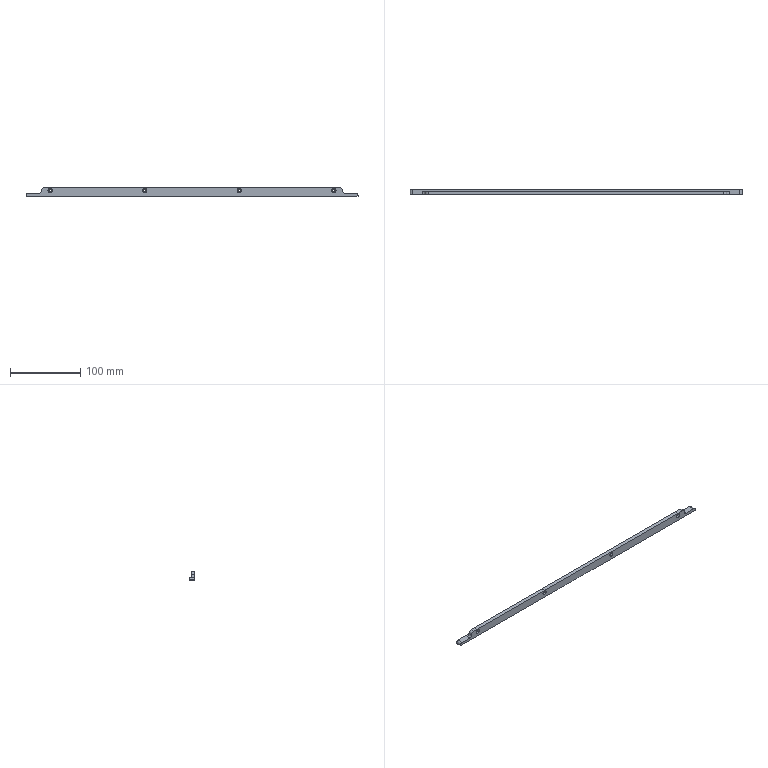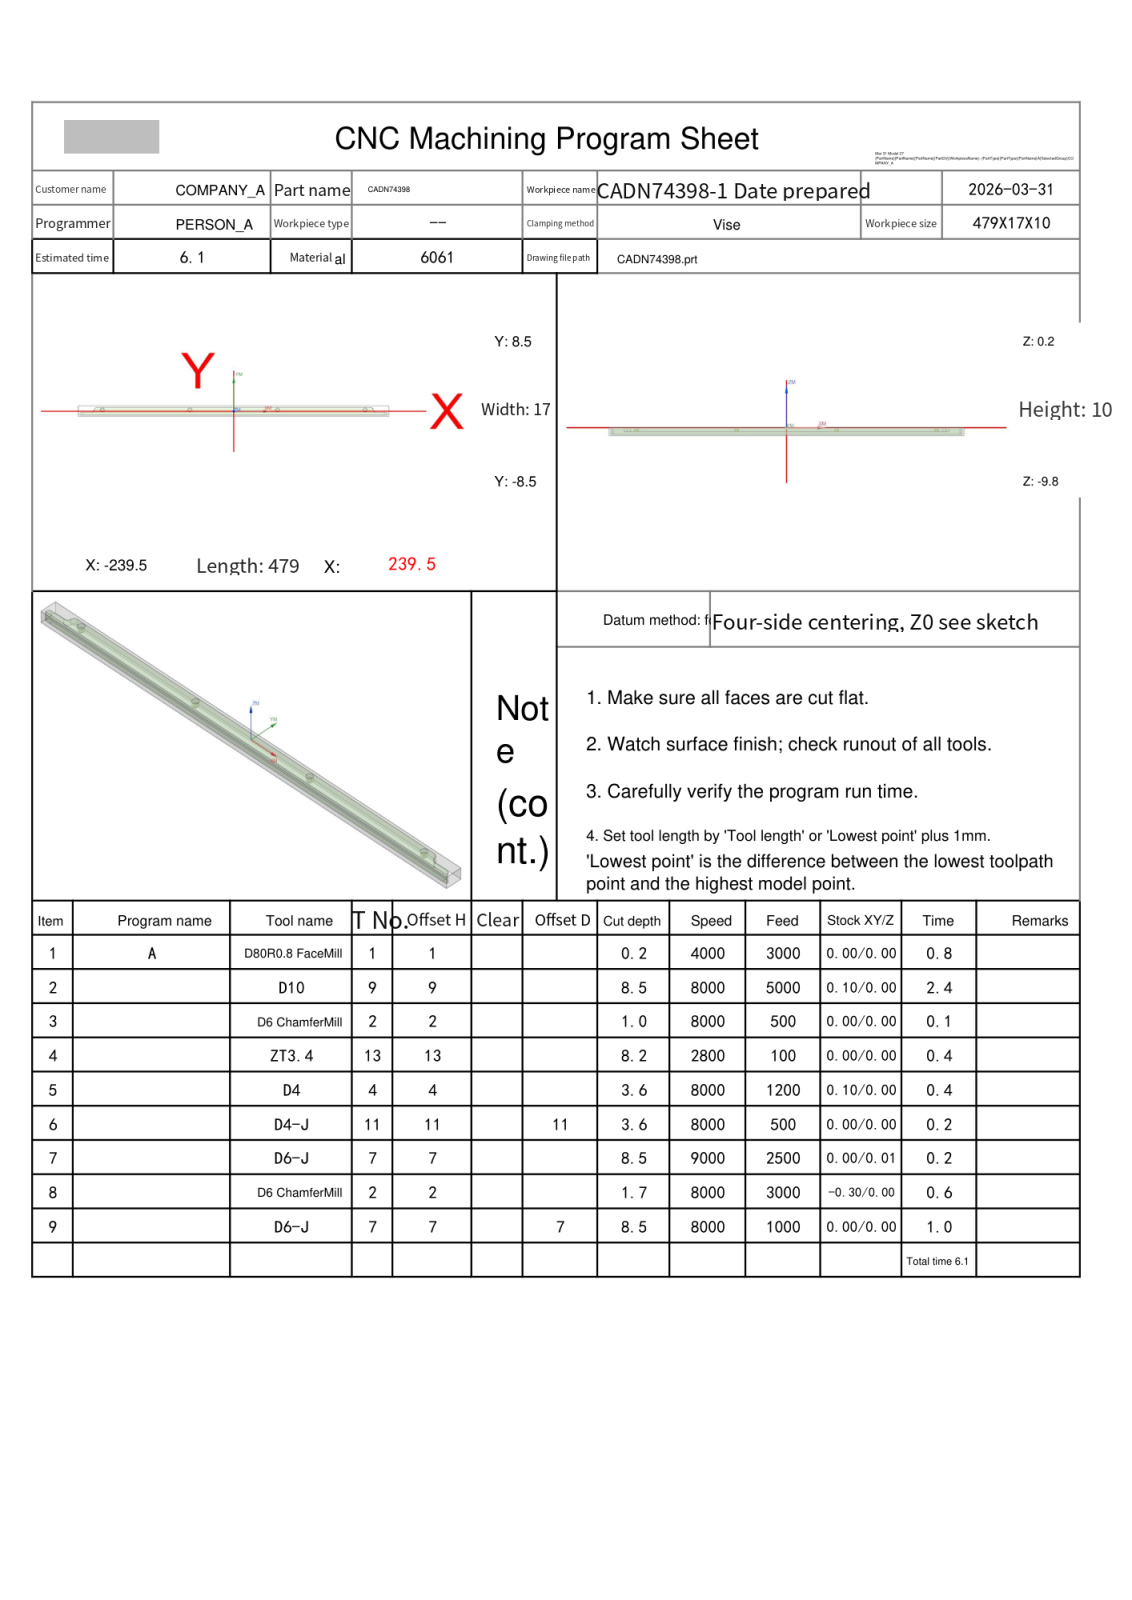NC program | NX | posted by the shop | part box 474 x 8.3 x 12 mm
Lines 413 to 2396 of 2396, first 1542 of 1984 lines:
N7 T07 M06
(D6-J  D=6. R=0. H=07 ce=0.00 di=0.01)
G00 G90 G54 X-220.761 Y1.9 M03 S9000
G43 H07 Z20.
M08
Z.605
G01 X-220.759 Y1.89 Z.477 F2000.
X-220.755 Y1.861 Z.36
X-220.746 Y1.817 Z.255
X-220.734 Y1.759 Z.161
X-220.718 Y1.691 Z.078
X-220.697 Y1.615 Z.004
X-220.672 Y1.534 Z-.06
X-220.641 Y1.45 Z-.115
X-220.604 Y1.366 Z-.161
X-220.562 Y1.285 Z-.2
X-220.513 Y1.209 Z-.231
X-220.457 Y1.141 Z-.255
X-220.394 Y1.083 Z-.273
X-220.324 Y1.039 Z-.286
X-220.247 Y1.01 Z-.292
X-220.161 Y1. Z-.295
X-219. F2500.
G03 X-218. Y2. I0.0 J1.
G02 X-217.924 Y3.026 I7. J0.0
G01 X-217.929 Y3.101 Z-.296
X-217.965 Y3.165 Z-.298
X-218.028 Y3.219 Z-.302
X-218.115 Y3.261 Z-.308
X-218.221 Y3.293 Z-.315
X-218.342 Y3.313 Z-.323
X-218.475 Y3.323 Z-.331
X-218.616 Z-.341
X-218.76 Y3.311 Z-.352
X-218.905 Y3.289 Z-.363
X-219.045 Y3.257 Z-.374
X-219.284 Y3.171 Z-.396
X-219.498 Y3.05 Z-.419
X-219.688 Y2.896 Z-.442
X-219.854 Y2.709 Z-.465
X-219.999 Y2.491 Z-.488
X-220.123 Y2.241 Z-.509
X-220.182 Y2.093 Z-.521
X-220.234 Y1.939 Z-.532
X-220.277 Y1.785 Z-.543
X-220.311 Y1.634 Z-.552
X-220.333 Y1.49 Z-.561
X-220.343 Y1.357 Z-.569
X-220.34 Y1.239 Z-.576
X-220.321 Y1.141 Z-.582
X-220.285 Y1.065 Z-.586
X-220.233 Y1.017 Z-.588
X-220.161 Y1. Z-.589
X-219.
G03 X-218. Y2. I0.0 J1.
G02 X-217.924 Y3.026 I7. J0.0
G01 X-217.929 Y3.101 Z-.59
X-217.965 Y3.165 Z-.593
X-218.028 Y3.219 Z-.597
X-218.115 Y3.261 Z-.602
X-218.221 Y3.293 Z-.609
X-218.342 Y3.313 Z-.617
X-218.475 Y3.323 Z-.626
X-218.616 Z-.636
X-218.76 Y3.311 Z-.646
X-218.905 Y3.289 Z-.658
X-219.045 Y3.257 Z-.669
X-219.284 Y3.171 Z-.691
X-219.498 Y3.05 Z-.714
X-219.688 Y2.896 Z-.737
X-219.854 Y2.709 Z-.76
X-219.999 Y2.491 Z-.782
X-220.123 Y2.241 Z-.804
X-220.182 Y2.093 Z-.816
X-220.234 Y1.939 Z-.827
X-220.277 Y1.785 Z-.837
X-220.311 Y1.634 Z-.847
X-220.333 Y1.49 Z-.856
X-220.343 Y1.357 Z-.864
X-220.34 Y1.239 Z-.871
X-220.321 Y1.141 Z-.876
X-220.285 Y1.065 Z-.88
X-220.233 Y1.017 Z-.883
X-220.161 Y1. Z-.884
X-219.
G03 X-218. Y2. I0.0 J1.
G02 X-217.924 Y3.026 I7. J0.0
G01 X-217.929 Y3.101 Z-.885
X-217.965 Y3.165 Z-.887
X-218.028 Y3.219 Z-.892
X-218.115 Y3.261 Z-.897
X-218.221 Y3.293 Z-.904
X-218.342 Y3.313 Z-.912
X-218.475 Y3.323 Z-.921
X-218.616 Z-.931
X-218.76 Y3.311 Z-.941
X-218.905 Y3.289 Z-.952
X-219.045 Y3.257 Z-.964
X-219.284 Y3.171 Z-.986
X-219.498 Y3.05 Z-1.008
X-219.688 Y2.896 Z-1.031
X-219.854 Y2.709 Z-1.054
X-219.999 Y2.491 Z-1.077
X-220.123 Y2.241 Z-1.099
X-220.182 Y2.093 Z-1.11
X-220.234 Y1.939 Z-1.121
X-220.277 Y1.785 Z-1.132
X-220.311 Y1.634 Z-1.142
X-220.333 Y1.49 Z-1.151
X-220.343 Y1.357 Z-1.159
X-220.34 Y1.239 Z-1.165
X-220.321 Y1.141 Z-1.171
X-220.285 Y1.065 Z-1.175
X-220.233 Y1.017 Z-1.178
X-220.161 Y1. Z-1.179
X-219.
G03 X-218. Y2. I0.0 J1.
G02 X-217.924 Y3.026 I7. J0.0
G01 X-217.929 Y3.101
X-217.965 Y3.165 Z-1.182
X-218.028 Y3.219 Z-1.186
X-218.115 Y3.261 Z-1.192
X-218.221 Y3.293 Z-1.199
X-218.342 Y3.313 Z-1.206
X-218.475 Y3.323 Z-1.215
X-218.616 Z-1.225
X-218.76 Y3.311 Z-1.236
X-218.905 Y3.289 Z-1.247
X-219.045 Y3.257 Z-1.258
X-219.284 Y3.171 Z-1.28
X-219.498 Y3.05 Z-1.303
X-219.688 Y2.896 Z-1.326
X-219.854 Y2.709 Z-1.349
X-219.999 Y2.491 Z-1.371
X-220.123 Y2.241 Z-1.393
X-220.182 Y2.093 Z-1.405
X-220.234 Y1.939 Z-1.416
X-220.277 Y1.785 Z-1.427
X-220.311 Y1.634 Z-1.436
X-220.333 Y1.49 Z-1.445
X-220.343 Y1.357 Z-1.453
X-220.34 Y1.239 Z-1.46
X-220.321 Y1.141 Z-1.466
X-220.285 Y1.065 Z-1.47
X-220.233 Y1.017 Z-1.472
X-220.161 Y1. Z-1.473
X-219.
G03 X-218. Y2. I0.0 J1.
G02 X-217.924 Y3.026 I7. J0.0
G01 X-217.929 Y3.101 Z-1.474
X-217.965 Y3.165 Z-1.477
X-218.028 Y3.219 Z-1.481
X-218.115 Y3.261 Z-1.486
X-218.221 Y3.293 Z-1.493
X-218.342 Y3.313 Z-1.501
X-218.475 Y3.323 Z-1.51
X-218.616 Z-1.52
X-218.76 Y3.311 Z-1.53
X-218.905 Y3.289 Z-1.541
X-219.045 Y3.257 Z-1.553
X-219.284 Y3.171 Z-1.575
X-219.498 Y3.05 Z-1.598
X-219.688 Y2.896 Z-1.621
X-219.854 Y2.709 Z-1.643
X-219.999 Y2.491 Z-1.666
X-220.123 Y2.241 Z-1.688
X-220.182 Y2.093 Z-1.7
X-220.234 Y1.939 Z-1.711
X-220.277 Y1.785 Z-1.721
X-220.311 Y1.634 Z-1.731
X-220.333 Y1.49 Z-1.74
X-220.343 Y1.357 Z-1.748
X-220.34 Y1.239 Z-1.755
X-220.321 Y1.141 Z-1.76
X-220.285 Y1.065 Z-1.764
X-220.233 Y1.017 Z-1.767
X-220.161 Y1. Z-1.768
X-219.
G03 X-218. Y2. I0.0 J1.
G02 X-217.924 Y3.026 I7. J0.0
G01 X-217.929 Y3.101 Z-1.769
X-217.965 Y3.165 Z-1.771
X-218.028 Y3.219 Z-1.775
X-218.115 Y3.261 Z-1.781
X-218.221 Y3.293 Z-1.788
X-218.342 Y3.313 Z-1.796
X-218.475 Y3.323 Z-1.805
X-218.616 Z-1.814
X-218.76 Y3.311 Z-1.825
X-218.905 Y3.289 Z-1.836
X-219.045 Y3.257 Z-1.848
X-219.284 Y3.171 Z-1.87
X-219.498 Y3.05 Z-1.892
X-219.688 Y2.896 Z-1.915
X-219.854 Y2.709 Z-1.938
X-219.999 Y2.491 Z-1.961
X-220.123 Y2.241 Z-1.983
X-220.182 Y2.093 Z-1.994
X-220.234 Y1.939 Z-2.005
X-220.277 Y1.785 Z-2.016
X-220.311 Y1.634 Z-2.026
X-220.333 Y1.49 Z-2.035
X-220.343 Y1.357 Z-2.043
X-220.34 Y1.239 Z-2.049
X-220.321 Y1.141 Z-2.055
X-220.285 Y1.065 Z-2.059
X-220.233 Y1.017 Z-2.062
X-220.161 Y1. Z-2.063
X-219.
G03 X-218. Y2. I0.0 J1.
G02 X-217.924 Y3.026 I7. J0.0
G01 X-217.929 Y3.101
X-217.965 Y3.165 Z-2.066
X-218.028 Y3.219 Z-2.07
X-218.115 Y3.261 Z-2.076
X-218.221 Y3.293 Z-2.082
X-218.342 Y3.313 Z-2.09
X-218.475 Y3.323 Z-2.099
X-218.616 Z-2.109
X-218.76 Y3.311 Z-2.12
X-218.905 Y3.289 Z-2.131
X-219.045 Y3.257 Z-2.142
X-219.284 Y3.171 Z-2.164
X-219.498 Y3.05 Z-2.187
X-219.688 Y2.896 Z-2.21
X-219.854 Y2.709 Z-2.233
X-219.999 Y2.491 Z-2.255
X-220.123 Y2.241 Z-2.277
X-220.182 Y2.093 Z-2.289
X-220.234 Y1.939 Z-2.3
X-220.277 Y1.785 Z-2.311
X-220.311 Y1.634 Z-2.32
X-220.333 Y1.49 Z-2.329
X-220.343 Y1.357 Z-2.337
X-220.34 Y1.239 Z-2.344
X-220.321 Y1.141 Z-2.35
X-220.285 Y1.065 Z-2.354
X-220.233 Y1.017 Z-2.356
X-220.161 Y1. Z-2.357
X-219.
G03 X-218. Y2. I0.0 J1.
G02 X-217.924 Y3.026 I7. J0.0
G01 X-217.929 Y3.101 Z-2.358
X-217.965 Y3.165 Z-2.361
X-218.028 Y3.219 Z-2.365
X-218.115 Y3.261 Z-2.37
X-218.221 Y3.293 Z-2.377
X-218.342 Y3.313 Z-2.385
X-218.475 Y3.323 Z-2.394
X-218.616 Z-2.404
X-218.76 Y3.311 Z-2.414
X-218.905 Y3.289 Z-2.425
X-219.045 Y3.257 Z-2.437
X-219.284 Y3.171 Z-2.459
X-219.498 Y3.05 Z-2.482
X-219.688 Y2.896 Z-2.504
X-219.854 Y2.709 Z-2.527
X-219.999 Y2.491 Z-2.55
X-220.123 Y2.241 Z-2.572
X-220.182 Y2.093 Z-2.584
X-220.234 Y1.939 Z-2.595
X-220.277 Y1.785 Z-2.605
X-220.311 Y1.634 Z-2.615
X-220.333 Y1.49 Z-2.624
X-220.343 Y1.357 Z-2.632
X-220.34 Y1.239 Z-2.639
X-220.321 Y1.141 Z-2.644
X-220.285 Y1.065 Z-2.648
X-220.233 Y1.017 Z-2.651
X-220.161 Y1. Z-2.652
X-219.
G03 X-218. Y2. I0.0 J1.
G02 X-217.924 Y3.026 I7. J0.0
G01 X-217.929 Y3.101 Z-2.653
X-217.965 Y3.165 Z-2.655
X-218.028 Y3.219 Z-2.659
X-218.115 Y3.261 Z-2.665
X-218.221 Y3.293 Z-2.672
X-218.342 Y3.313 Z-2.68
X-218.475 Y3.323 Z-2.689
X-218.616 Z-2.698
X-218.76 Y3.311 Z-2.709
X-218.905 Y3.289 Z-2.72
X-219.045 Y3.257 Z-2.732
X-219.284 Y3.171 Z-2.754
X-219.498 Y3.05 Z-2.776
X-219.688 Y2.896 Z-2.799
X-219.854 Y2.709 Z-2.822
X-219.999 Y2.491 Z-2.845
X-220.123 Y2.241 Z-2.867
X-220.182 Y2.093 Z-2.878
X-220.234 Y1.939 Z-2.889
X-220.277 Y1.785 Z-2.9
X-220.311 Y1.634 Z-2.91
X-220.333 Y1.49 Z-2.919
X-220.343 Y1.357 Z-2.926
X-220.34 Y1.239 Z-2.933
X-220.321 Y1.141 Z-2.939
X-220.285 Y1.065 Z-2.943
X-220.233 Y1.017 Z-2.946
X-220.161 Y1.
X-219.
G03 X-218. Y2. I0.0 J1.
G02 X-217.924 Y3.026 I7. J0.0
G01 X-217.929 Y3.101 Z-2.947
X-217.965 Y3.165 Z-2.95
X-218.028 Y3.219 Z-2.954
X-218.115 Y3.261 Z-2.96
X-218.221 Y3.293 Z-2.966
X-218.342 Y3.313 Z-2.974
X-218.475 Y3.323 Z-2.983
X-218.616 Z-2.993
X-218.76 Y3.311 Z-3.004
X-218.905 Y3.289 Z-3.015
X-219.045 Y3.257 Z-3.026
X-219.284 Y3.171 Z-3.048
X-219.498 Y3.05 Z-3.071
X-219.688 Y2.896 Z-3.094
X-219.854 Y2.709 Z-3.117
X-219.999 Y2.491 Z-3.139
X-220.123 Y2.241 Z-3.161
X-220.182 Y2.093 Z-3.173
X-220.234 Y1.939 Z-3.184
X-220.277 Y1.785 Z-3.194
X-220.311 Y1.634 Z-3.204
X-220.333 Y1.49 Z-3.213
X-220.343 Y1.357 Z-3.221
X-220.34 Y1.239 Z-3.228
X-220.321 Y1.141 Z-3.233
X-220.285 Y1.065 Z-3.238
X-220.233 Y1.017 Z-3.24
X-220.161 Y1. Z-3.241
X-219.
G03 X-218. Y2. I0.0 J1.
G02 X-217.924 Y3.026 I7. J0.0
G01 X-217.929 Y3.101 Z-3.242
X-217.965 Y3.165 Z-3.245
X-218.028 Y3.219 Z-3.249
X-218.115 Y3.261 Z-3.254
X-218.221 Y3.293 Z-3.261
X-218.342 Y3.313 Z-3.269
X-218.475 Y3.323 Z-3.278
X-218.616 Z-3.288
X-218.76 Y3.311 Z-3.298
X-218.905 Y3.289 Z-3.309
X-219.045 Y3.257 Z-3.321
X-219.284 Y3.171 Z-3.343
X-219.498 Y3.05 Z-3.365
X-219.688 Y2.896 Z-3.388
X-219.854 Y2.709 Z-3.411
X-219.999 Y2.491 Z-3.434
X-220.123 Y2.241 Z-3.456
X-220.182 Y2.093 Z-3.467
X-220.234 Y1.939 Z-3.479
X-220.277 Y1.785 Z-3.489
X-220.311 Y1.634 Z-3.499
X-220.333 Y1.49 Z-3.508
X-220.343 Y1.357 Z-3.516
X-220.34 Y1.239 Z-3.523
X-220.321 Y1.141 Z-3.528
X-220.285 Y1.065 Z-3.532
X-220.233 Y1.017 Z-3.535
X-220.161 Y1. Z-3.536
X-219.
G03 X-218. Y2. I0.0 J1.
G02 X-217.924 Y3.026 I7. J0.0
G01 X-217.929 Y3.101 Z-3.537
X-217.965 Y3.165 Z-3.539
X-218.028 Y3.219 Z-3.543
X-218.115 Y3.261 Z-3.549
X-218.221 Y3.293 Z-3.556
X-218.342 Y3.313 Z-3.564
X-218.475 Y3.323 Z-3.573
X-218.616 Z-3.582
X-218.76 Y3.311 Z-3.593
X-218.905 Y3.289 Z-3.604
X-219.045 Y3.257 Z-3.616
X-219.284 Y3.171 Z-3.637
X-219.498 Y3.05 Z-3.66
X-219.688 Y2.896 Z-3.683
X-219.854 Y2.709 Z-3.706
X-219.999 Y2.491 Z-3.729
X-220.123 Y2.241 Z-3.751
X-220.182 Y2.093 Z-3.762
X-220.234 Y1.939 Z-3.773
X-220.277 Y1.785 Z-3.784
X-220.311 Y1.634 Z-3.794
X-220.333 Y1.49 Z-3.802
X-220.343 Y1.357 Z-3.81
X-220.34 Y1.239 Z-3.817
X-220.321 Y1.141 Z-3.823
X-220.285 Y1.065 Z-3.827
X-220.233 Y1.017 Z-3.829
X-220.161 Y1. Z-3.83
X-219.
G03 X-218. Y2. I0.0 J1.
G02 X-217.924 Y3.026 I7. J0.0
G01 X-217.929 Y3.101 Z-3.831
X-217.965 Y3.165 Z-3.834
X-218.028 Y3.219 Z-3.838
X-218.115 Y3.261 Z-3.843
X-218.221 Y3.293 Z-3.85
X-218.342 Y3.313 Z-3.858
X-218.475 Y3.323 Z-3.867
X-218.616 Z-3.877
X-218.76 Y3.311 Z-3.888
X-218.905 Y3.289 Z-3.899
X-219.045 Y3.257 Z-3.91
X-219.284 Y3.171 Z-3.932
X-219.498 Y3.05 Z-3.955
X-219.688 Y2.896 Z-3.978
X-219.854 Y2.709 Z-4.001
X-219.999 Y2.491 Z-4.023
X-220.123 Y2.241 Z-4.045
X-220.182 Y2.093 Z-4.057
X-220.234 Y1.939 Z-4.068
X-220.277 Y1.785 Z-4.078
X-220.311 Y1.634 Z-4.088
X-220.333 Y1.49 Z-4.097
X-220.343 Y1.357 Z-4.105
X-220.34 Y1.239 Z-4.112
X-220.321 Y1.141 Z-4.117
X-220.285 Y1.065 Z-4.122
X-220.233 Y1.017 Z-4.124
X-220.161 Y1. Z-4.125
X-219.
G03 X-218. Y2. I0.0 J1.
G02 X-217.924 Y3.026 I7. J0.0
G01 X-217.929 Y3.101 Z-4.126
X-217.965 Y3.165 Z-4.128
X-218.028 Y3.219 Z-4.133
X-218.115 Y3.261 Z-4.138
X-218.221 Y3.293 Z-4.145
X-218.342 Y3.313 Z-4.153
X-218.475 Y3.323 Z-4.162
X-218.616 Z-4.172
X-218.76 Y3.311 Z-4.182
X-218.905 Y3.289 Z-4.193
X-219.045 Y3.257 Z-4.205
X-219.284 Y3.171 Z-4.227
X-219.498 Y3.05 Z-4.249
X-219.688 Y2.896 Z-4.272
X-219.854 Y2.709 Z-4.295
X-219.999 Y2.491 Z-4.318
X-220.123 Y2.241 Z-4.34
X-220.182 Y2.093 Z-4.351
X-220.234 Y1.939 Z-4.362
X-220.277 Y1.785 Z-4.373
X-220.311 Y1.634 Z-4.383
X-220.333 Y1.49 Z-4.392
X-220.343 Y1.357 Z-4.4
X-220.34 Y1.239 Z-4.407
X-220.321 Y1.141 Z-4.412
X-220.285 Y1.065 Z-4.416
X-220.233 Y1.017 Z-4.419
X-220.161 Y1. Z-4.42
X-219.
G03 X-218. Y2. I0.0 J1.
G02 X-217.924 Y3.026 I7. J0.0
G01 X-217.929 Y3.101 Z-4.421
X-217.965 Y3.165 Z-4.423
X-218.028 Y3.219 Z-4.427
X-218.115 Y3.261 Z-4.433
X-218.221 Y3.293 Z-4.44
X-218.342 Y3.313 Z-4.448
X-218.475 Y3.323 Z-4.456
X-218.616 Z-4.466
X-218.76 Y3.311 Z-4.477
X-218.905 Y3.289 Z-4.488
X-219.045 Y3.257 Z-4.499
X-219.284 Y3.171 Z-4.521
X-219.498 Y3.05 Z-4.544
X-219.688 Y2.896 Z-4.567
X-219.854 Y2.709 Z-4.59
X-219.999 Y2.491 Z-4.613
X-220.123 Y2.241 Z-4.634
X-220.182 Y2.093 Z-4.646
X-220.234 Y1.939 Z-4.657
X-220.277 Y1.785 Z-4.668
X-220.311 Y1.634 Z-4.677
X-220.333 Y1.49 Z-4.686
X-220.343 Y1.357 Z-4.694
X-220.34 Y1.239 Z-4.701
X-220.321 Y1.141 Z-4.707
X-220.285 Y1.065 Z-4.711
X-220.233 Y1.017 Z-4.713
X-220.161 Y1. Z-4.714
X-219.
G03 X-218. Y2. I0.0 J1.
G02 X-217.924 Y3.026 I7. J0.0
G01 X-217.929 Y3.101 Z-4.715
X-217.965 Y3.165 Z-4.718
X-218.028 Y3.219 Z-4.722
X-218.115 Y3.261 Z-4.727
X-218.221 Y3.293 Z-4.734
X-218.342 Y3.313 Z-4.742
X-218.475 Y3.323 Z-4.751
X-218.616 Z-4.761
X-218.76 Y3.311 Z-4.771
X-218.905 Y3.289 Z-4.783
X-219.046 Y3.257 Z-4.794
X-219.284 Y3.171 Z-4.816
X-219.498 Y3.05 Z-4.839
X-219.688 Y2.896 Z-4.862
X-219.855 Y2.709 Z-4.885
X-219.999 Y2.491 Z-4.907
X-220.123 Y2.241 Z-4.929
X-220.182 Y2.093 Z-4.941
X-220.234 Y1.939 Z-4.952
X-220.278 Y1.785 Z-4.962
X-220.311 Y1.634 Z-4.972
X-220.334 Y1.49 Z-4.981
X-220.344 Y1.357 Z-4.989
X-220.34 Y1.239 Z-4.996
X-220.321 Y1.141 Z-5.001
X-220.286 Y1.065 Z-5.005
X-220.233 Y1.017 Z-5.008
X-220.161 Y1. Z-5.009
X-219.
G03 X-218. Y2. I0.0 J1.
G02 X-217.924 Y3.028 I7. J0.0
G01 X-217.929 Y3.103 Z-5.01
X-217.965 Y3.168 Z-5.012
X-218.028 Y3.221 Z-5.017
X-218.114 Y3.263 Z-5.022
X-218.22 Y3.295 Z-5.029
X-218.342 Y3.316 Z-5.037
X-218.475 Y3.325 Z-5.046
X-218.615 Z-5.056
X-218.76 Y3.313 Z-5.066
X-218.904 Y3.291 Z-5.077
X-219.045 Y3.259 Z-5.089
X-219.284 Y3.172 Z-5.111
X-219.498 Y3.051 Z-5.133
X-219.688 Y2.897 Z-5.156
X-219.854 Y2.71 Z-5.179
X-219.999 Y2.491 Z-5.202
X-220.123 Y2.242 Z-5.224
X-220.182 Y2.093 Z-5.235
X-220.234 Y1.94 Z-5.246
X-220.278 Y1.786 Z-5.257
X-220.311 Y1.634 Z-5.267
X-220.334 Y1.49 Z-5.276
X-220.344 Y1.357 Z-5.284
X-220.34 Y1.239 Z-5.29
X-220.321 Y1.141 Z-5.296
X-220.286 Y1.065 Z-5.3
X-220.233 Y1.017 Z-5.303
X-220.161 Y1. Z-5.304
X-219.
G03 X-218. Y2. I0.0 J1.
G02 X-217.924 Y3.028 I7. J0.0
G01 X-217.929 Y3.103
X-217.965 Y3.168 Z-5.307
X-218.028 Y3.221 Z-5.311
X-218.114 Y3.263 Z-5.317
X-218.22 Y3.295 Z-5.324
X-218.342 Y3.316 Z-5.331
X-218.475 Y3.325 Z-5.34
X-218.615 Z-5.35
X-218.76 Y3.313 Z-5.361
X-218.904 Y3.291 Z-5.372
X-219.045 Y3.259 Z-5.383
X-219.284 Y3.172 Z-5.405
X-219.498 Y3.051 Z-5.428
X-219.688 Y2.897 Z-5.451
X-219.854 Y2.71 Z-5.474
X-219.999 Y2.491 Z-5.496
X-220.123 Y2.242 Z-5.518
X-220.182 Y2.093 Z-5.53
X-220.234 Y1.94 Z-5.541
X-220.278 Y1.786 Z-5.552
X-220.311 Y1.634 Z-5.561
X-220.334 Y1.49 Z-5.57
X-220.344 Y1.357 Z-5.578
X-220.34 Y1.239 Z-5.585
X-220.321 Y1.141 Z-5.591
X-220.286 Y1.065 Z-5.595
X-220.233 Y1.017 Z-5.597
X-220.161 Y1. Z-5.598
X-219.
G03 X-218. Y2. I0.0 J1.
G02 X-217.924 Y3.028 I7. J0.0
G01 X-217.929 Y3.103 Z-5.599
X-217.965 Y3.168 Z-5.602
X-218.028 Y3.221 Z-5.606
X-218.114 Y3.263 Z-5.611
X-218.22 Y3.295 Z-5.618
X-218.342 Y3.316 Z-5.626
X-218.475 Y3.325 Z-5.635
X-218.615 Z-5.645
X-218.76 Y3.313 Z-5.655
X-218.904 Y3.291 Z-5.666
X-219.045 Y3.259 Z-5.678
X-219.284 Y3.172 Z-5.7
X-219.498 Y3.051 Z-5.723
X-219.688 Y2.897 Z-5.746
X-219.854 Y2.71 Z-5.768
X-219.999 Y2.491 Z-5.791
X-220.123 Y2.242 Z-5.813
X-220.182 Y2.093 Z-5.825
X-220.234 Y1.94 Z-5.836
X-220.278 Y1.786 Z-5.846
X-220.311 Y1.634 Z-5.856
X-220.334 Y1.49 Z-5.865
X-220.344 Y1.357 Z-5.873
X-220.34 Y1.239 Z-5.88
X-220.321 Y1.141 Z-5.885
X-220.286 Y1.065 Z-5.889
X-220.233 Y1.017 Z-5.892
X-220.161 Y1. Z-5.893
X-219.
G03 X-218. Y2. I0.0 J1.
G02 X-217.924 Y3.028 I7. J0.0
G01 X-217.929 Y3.103 Z-5.894
X-217.965 Y3.168 Z-5.896
X-218.028 Y3.221 Z-5.9
X-218.114 Y3.263 Z-5.906
X-218.22 Y3.295 Z-5.913
X-218.342 Y3.316 Z-5.921
X-218.475 Y3.325 Z-5.93
X-218.615 Z-5.939
X-218.76 Y3.313 Z-5.95
X-218.904 Y3.291 Z-5.961
X-219.045 Y3.259 Z-5.973
X-219.284 Y3.172 Z-5.995
X-219.498 Y3.051 Z-6.017
X-219.688 Y2.897 Z-6.04
X-219.854 Y2.71 Z-6.063
X-219.999 Y2.491 Z-6.086
X-220.123 Y2.242 Z-6.108
X-220.182 Y2.093 Z-6.119
X-220.234 Y1.94 Z-6.13
X-220.278 Y1.786 Z-6.141
X-220.311 Y1.634 Z-6.151
X-220.334 Y1.49 Z-6.16
X-220.344 Y1.357 Z-6.168
X-220.34 Y1.239 Z-6.174
X-220.321 Y1.141 Z-6.18
X-220.286 Y1.065 Z-6.184
X-220.233 Y1.017 Z-6.187
X-220.161 Y1. Z-6.188
X-219.
G03 X-218. Y2. I0.0 J1.
G02 X-217.924 Y3.028 I7. J0.0
G01 X-217.929 Y3.103
X-217.965 Y3.168 Z-6.191
X-218.028 Y3.221 Z-6.195
X-218.114 Y3.263 Z-6.201
X-218.22 Y3.295 Z-6.207
X-218.342 Y3.316 Z-6.215
X-218.475 Y3.325 Z-6.224
X-218.615 Z-6.234
X-218.76 Y3.313 Z-6.245
X-218.904 Y3.291 Z-6.256
X-219.045 Y3.259 Z-6.267
X-219.284 Y3.172 Z-6.289
X-219.498 Y3.051 Z-6.312
X-219.688 Y2.897 Z-6.335
X-219.854 Y2.71 Z-6.358
X-219.999 Y2.491 Z-6.38
X-220.123 Y2.242 Z-6.402
X-220.182 Y2.093 Z-6.414
X-220.234 Y1.94 Z-6.425
X-220.278 Y1.786 Z-6.436
X-220.311 Y1.634 Z-6.445
X-220.334 Y1.49 Z-6.454
X-220.344 Y1.357 Z-6.462
X-220.34 Y1.239 Z-6.469
X-220.321 Y1.141 Z-6.475
X-220.286 Y1.065 Z-6.479
X-220.233 Y1.017 Z-6.481
X-220.161 Y1. Z-6.482
X-219.
G03 X-218. Y2. I0.0 J1.
G02 X-217.924 Y3.028 I7. J0.0
G01 X-217.929 Y3.103 Z-6.483
X-217.965 Y3.168 Z-6.486
X-218.028 Y3.221 Z-6.49
X-218.114 Y3.263 Z-6.495
X-218.22 Y3.295 Z-6.502
X-218.342 Y3.316 Z-6.51
X-218.475 Y3.325 Z-6.519
X-218.615 Z-6.529
X-218.76 Y3.313 Z-6.539
X-218.904 Y3.291 Z-6.55
X-219.045 Y3.259 Z-6.562
X-219.284 Y3.172 Z-6.584
X-219.498 Y3.051 Z-6.607
X-219.688 Y2.897 Z-6.629
X-219.854 Y2.71 Z-6.652
X-219.999 Y2.491 Z-6.675
X-220.123 Y2.242 Z-6.697
X-220.182 Y2.093 Z-6.709
X-220.234 Y1.94 Z-6.72
X-220.278 Y1.786 Z-6.73
X-220.311 Y1.634 Z-6.74
X-220.334 Y1.49 Z-6.749
X-220.344 Y1.357 Z-6.757
X-220.34 Y1.239 Z-6.764
X-220.321 Y1.141 Z-6.769
X-220.286 Y1.065 Z-6.773
X-220.233 Y1.017 Z-6.776
X-220.161 Y1. Z-6.777
X-219.
G03 X-218. Y2. I0.0 J1.
G02 X-217.924 Y3.028 I7. J0.0
G01 X-217.929 Y3.103 Z-6.778
X-217.965 Y3.168 Z-6.78
X-218.028 Y3.221 Z-6.784
X-218.114 Y3.263 Z-6.79
X-218.22 Y3.295 Z-6.797
X-218.342 Y3.316 Z-6.805
X-218.475 Y3.325 Z-6.814
X-218.615 Z-6.823
X-218.76 Y3.313 Z-6.834
X-218.904 Y3.291 Z-6.845
X-219.045 Y3.259 Z-6.857
X-219.284 Y3.172 Z-6.879
X-219.498 Y3.051 Z-6.901
X-219.688 Y2.897 Z-6.924
X-219.854 Y2.71 Z-6.947
X-219.999 Y2.491 Z-6.97
X-220.123 Y2.242 Z-6.992
X-220.182 Y2.093 Z-7.003
X-220.234 Y1.94 Z-7.014
X-220.278 Y1.786 Z-7.025
X-220.311 Y1.634 Z-7.035
X-220.334 Y1.49 Z-7.044
X-220.344 Y1.357 Z-7.051
X-220.34 Y1.239 Z-7.058
X-220.321 Y1.141 Z-7.064
X-220.286 Y1.065 Z-7.068
X-220.233 Y1.017 Z-7.071
X-220.161 Y1.
X-219.
G03 X-218. Y2. I0.0 J1.
G02 X-217.924 Y3.028 I7. J0.0
G01 X-217.929 Y3.103 Z-7.072
X-217.965 Y3.168 Z-7.075
X-218.028 Y3.221 Z-7.079
X-218.114 Y3.263 Z-7.085
X-218.22 Y3.295 Z-7.091
X-218.342 Y3.316 Z-7.099
X-218.475 Y3.325 Z-7.108
X-218.615 Z-7.118
X-218.76 Y3.313 Z-7.129
X-218.904 Y3.291 Z-7.14
X-219.045 Y3.259 Z-7.151
X-219.284 Y3.172 Z-7.173
X-219.498 Y3.051 Z-7.196
X-219.688 Y2.897 Z-7.219
X-219.854 Y2.71 Z-7.242
X-219.999 Y2.491 Z-7.264
X-220.123 Y2.242 Z-7.286
X-220.182 Y2.093 Z-7.298
X-220.234 Y1.94 Z-7.309
X-220.278 Y1.786 Z-7.319
X-220.311 Y1.634 Z-7.329
X-220.334 Y1.49 Z-7.338
X-220.344 Y1.357 Z-7.346
X-220.34 Y1.239 Z-7.353
X-220.321 Y1.141 Z-7.358
X-220.286 Y1.065 Z-7.363
X-220.233 Y1.017 Z-7.365
X-220.161 Y1. Z-7.366
X-219.
G03 X-218. Y2. I0.0 J1.
G02 X-217.924 Y3.028 I7. J0.0
G01 X-217.929 Y3.103 Z-7.367
X-217.965 Y3.168 Z-7.37
X-218.028 Y3.221 Z-7.374
X-218.114 Y3.263 Z-7.379
X-218.22 Y3.295 Z-7.386
X-218.342 Y3.316 Z-7.394
X-218.475 Y3.325 Z-7.403
X-218.615 Z-7.413
X-218.76 Y3.313 Z-7.423
X-218.904 Y3.291 Z-7.434
X-219.045 Y3.259 Z-7.446
X-219.284 Y3.172 Z-7.468
X-219.498 Y3.051 Z-7.49
X-219.688 Y2.897 Z-7.513
X-219.854 Y2.71 Z-7.536
X-219.999 Y2.491 Z-7.559
X-220.123 Y2.242 Z-7.581
X-220.182 Y2.093 Z-7.592
X-220.234 Y1.94 Z-7.604
X-220.278 Y1.786 Z-7.614
X-220.311 Y1.634 Z-7.624
X-220.334 Y1.49 Z-7.633
X-220.344 Y1.357 Z-7.641
X-220.34 Y1.239 Z-7.648
X-220.321 Y1.141 Z-7.653
X-220.286 Y1.065 Z-7.657
X-220.233 Y1.017 Z-7.66
X-220.161 Y1. Z-7.661
X-219.
G03 X-218. Y2. I0.0 J1.
G02 X-217.924 Y3.028 I7. J0.0
G01 X-217.929 Y3.103 Z-7.662
X-217.965 Y3.168 Z-7.664
X-218.028 Y3.221 Z-7.668
X-218.114 Y3.263 Z-7.674
X-218.22 Y3.295 Z-7.681
X-218.342 Y3.316 Z-7.689
X-218.475 Y3.326 Z-7.698
X-218.615 Y3.325 Z-7.707
X-218.76 Y3.313 Z-7.718
X-218.904 Y3.292 Z-7.729
X-219.045 Y3.259 Z-7.741
X-219.284 Y3.173 Z-7.762
X-219.498 Y3.052 Z-7.785
X-219.688 Y2.898 Z-7.808
X-219.854 Y2.711 Z-7.831
X-219.999 Y2.492 Z-7.854
X-220.123 Y2.242 Z-7.876
X-220.182 Y2.094 Z-7.887
X-220.234 Y1.94 Z-7.898
X-220.278 Y1.786 Z-7.909
X-220.311 Y1.635 Z-7.919
X-220.334 Y1.49 Z-7.927
X-220.344 Y1.357 Z-7.935
X-220.34 Y1.239 Z-7.942
X-220.321 Y1.141 Z-7.948
X-220.286 Y1.065 Z-7.952
X-220.233 Y1.017 Z-7.954
X-220.161 Y1. Z-7.955
X-219.
G03 X-218. Y2. I0.0 J1.
G02 X-217.924 Y3.028 I7. J0.0
G01 X-217.929 Y3.103 Z-7.956
X-217.965 Y3.168 Z-7.959
X-218.028 Y3.221 Z-7.963
X-218.114 Y3.263 Z-7.968
X-218.22 Y3.295 Z-7.975
X-218.342 Y3.316 Z-7.983
X-218.475 Y3.326 Z-7.992
X-218.615 Y3.325 Z-8.002
X-218.76 Y3.313 Z-8.013
X-218.904 Y3.292 Z-8.024
X-219.045 Y3.259 Z-8.035
X-219.284 Y3.173 Z-8.057
X-219.498 Y3.052 Z-8.08
X-219.688 Y2.898 Z-8.103
X-219.854 Y2.711 Z-8.126
X-219.999 Y2.492 Z-8.148
X-220.123 Y2.242 Z-8.17
X-220.182 Y2.094 Z-8.182
X-220.234 Y1.94 Z-8.193
X-220.278 Y1.786 Z-8.203
X-220.311 Y1.635 Z-8.213
X-220.334 Y1.49 Z-8.222
X-220.344 Y1.357 Z-8.23
X-220.34 Y1.239 Z-8.237
X-220.321 Y1.141 Z-8.242
X-220.286 Y1.065 Z-8.247
X-220.233 Y1.017 Z-8.249
X-220.161 Y1. Z-8.25
X-219.
G03 X-218. Y2. I0.0 J1.
G02 X-217.924 Y3.028 I7. J0.0
G01 X-217.921 Y3.123 Z-8.247
X-217.94 Y3.218 Z-8.24
X-217.976 Y3.311 Z-8.226
X-218.027 Y3.401 Z-8.205
X-218.09 Y3.489 Z-8.177
X-218.161 Y3.573 Z-8.141
X-218.238 Y3.651 Z-8.096
X-218.317 Y3.724 Z-8.042
X-218.396 Y3.79 Z-7.978
X-218.471 Y3.848 Z-7.903
X-218.539 Y3.897 Z-7.818
X-218.597 Y3.938 Z-7.72
X-218.643 Y3.967 Z-7.61
X-218.672 Y3.986 Z-7.487
X-218.683 Y3.992 Z-7.35
G00 Z20.
X218.726 Y3.761
Z.605
G01 X218.716 Y3.758 Z.477 F2000.
X218.689 Y3.749 Z.36
X218.646 Y3.734 Z.255
X218.591 Y3.713 Z.161
X218.526 Y3.686 Z.078
X218.454 Y3.654 Z.004
X218.377 Y3.616 Z-.06
X218.299 Y3.572 Z-.115
X218.221 Y3.522 Z-.161
X218.147 Y3.467 Z-.2
X218.079 Y3.407 Z-.231
X218.02 Y3.341 Z-.255
X217.972 Y3.27 Z-.273
X217.939 Y3.194 Z-.286
X217.922 Y3.112 Z-.292
X217.924 Y3.026 Z-.295
G02 X218. Y2. I-6.924 J-1.026 F2500.
G03 X219. Y1. I1. J0.0
G01 X220.161
X220.234 Y1.016 Z-.296
X220.29 Y1.063 Z-.298
X220.33 Y1.135 Z-.302
X220.355 Y1.229 Z-.308
X220.365 Y1.342 Z-.315
X220.363 Y1.469 Z-.323
X220.348 Y1.606 Z-.331
X220.323 Y1.75 Z-.341
X220.287 Y1.896 Z-.352
X220.241 Y2.04 Z-.363
X220.188 Y2.18 Z-.374
X220.07 Y2.413 Z-.396
X219.928 Y2.616 Z-.419
X219.76 Y2.79 Z-.442
X219.565 Y2.936 Z-.465
X219.344 Y3.055 Z-.488
X219.096 Y3.148 Z-.509
X218.949 Y3.188 Z-.521
X218.799 Y3.22 Z-.532
X218.648 Y3.244 Z-.543
X218.501 Y3.258 Z-.552
X218.362 Y3.261 Z-.561
X218.235 Y3.254 Z-.569
X218.125 Y3.235 Z-.576
X218.034 Y3.203 Z-.582
X217.968 Y3.158 Z-.586
X217.93 Y3.099 Z-.588
X217.924 Y3.026 Z-.589
G02 X218. Y2. I-6.924 J-1.026
G03 X219. Y1. I1. J0.0
G01 X220.161
X220.234 Y1.016 Z-.59
X220.29 Y1.063 Z-.593
X220.33 Y1.135 Z-.597
X220.355 Y1.229 Z-.602
X220.365 Y1.342 Z-.609
X220.363 Y1.469 Z-.617
X220.348 Y1.606 Z-.626
X220.323 Y1.75 Z-.636
X220.287 Y1.896 Z-.646
X220.241 Y2.04 Z-.658
X220.188 Y2.18 Z-.669
X220.07 Y2.413 Z-.691
X219.928 Y2.616 Z-.714
X219.76 Y2.79 Z-.737
X219.565 Y2.936 Z-.76
X219.344 Y3.055 Z-.782
X219.096 Y3.148 Z-.804
X218.949 Y3.188 Z-.816
X218.799 Y3.22 Z-.827
X218.648 Y3.244 Z-.837
X218.501 Y3.258 Z-.847
X218.362 Y3.261 Z-.856
X218.235 Y3.254 Z-.864
X218.125 Y3.235 Z-.871
X218.034 Y3.203 Z-.876
X217.968 Y3.158 Z-.88
X217.93 Y3.099 Z-.883
X217.924 Y3.026 Z-.884
G02 X218. Y2. I-6.924 J-1.026
G03 X219. Y1. I1. J0.0
G01 X220.161
X220.234 Y1.016 Z-.885
X220.29 Y1.063 Z-.887
X220.33 Y1.135 Z-.892
X220.355 Y1.229 Z-.897
X220.365 Y1.342 Z-.904
X220.363 Y1.469 Z-.912
X220.348 Y1.606 Z-.921
X220.323 Y1.75 Z-.931
X220.287 Y1.896 Z-.941
X220.241 Y2.04 Z-.952
X220.188 Y2.18 Z-.964
X220.07 Y2.413 Z-.986
X219.928 Y2.616 Z-1.008
X219.76 Y2.79 Z-1.031
X219.565 Y2.936 Z-1.054
X219.344 Y3.055 Z-1.077
X219.096 Y3.148 Z-1.099
X218.949 Y3.188 Z-1.11
X218.799 Y3.22 Z-1.121
X218.648 Y3.244 Z-1.132
X218.501 Y3.258 Z-1.142
X218.362 Y3.261 Z-1.151
X218.235 Y3.254 Z-1.159
X218.125 Y3.235 Z-1.165
X218.034 Y3.203 Z-1.171
X217.968 Y3.158 Z-1.175
X217.93 Y3.099 Z-1.178
X217.924 Y3.026 Z-1.179
G02 X218. Y2. I-6.924 J-1.026
G03 X219. Y1. I1. J0.0
G01 X220.161
X220.234 Y1.016
X220.29 Y1.063 Z-1.182
X220.33 Y1.135 Z-1.186
X220.355 Y1.229 Z-1.192
X220.365 Y1.342 Z-1.199
X220.363 Y1.469 Z-1.206
X220.348 Y1.606 Z-1.215
X220.323 Y1.75 Z-1.225
X220.287 Y1.896 Z-1.236
X220.241 Y2.04 Z-1.247
X220.188 Y2.18 Z-1.258
X220.07 Y2.413 Z-1.28
X219.928 Y2.616 Z-1.303
X219.76 Y2.79 Z-1.326
X219.565 Y2.936 Z-1.349
X219.344 Y3.055 Z-1.371
X219.096 Y3.148 Z-1.393
X218.949 Y3.188 Z-1.405
X218.799 Y3.22 Z-1.416
X218.648 Y3.244 Z-1.427
X218.501 Y3.258 Z-1.436
X218.362 Y3.261 Z-1.445
X218.235 Y3.254 Z-1.453
X218.125 Y3.235 Z-1.46
X218.034 Y3.203 Z-1.466
X217.968 Y3.158 Z-1.47
X217.93 Y3.099 Z-1.472
X217.924 Y3.026 Z-1.473
G02 X218. Y2. I-6.924 J-1.026
G03 X219. Y1. I1. J0.0
G01 X220.161
X220.234 Y1.016 Z-1.474
X220.29 Y1.063 Z-1.477
X220.33 Y1.135 Z-1.481
X220.355 Y1.229 Z-1.486
X220.365 Y1.342 Z-1.493
X220.363 Y1.469 Z-1.501
X220.348 Y1.606 Z-1.51
X220.323 Y1.75 Z-1.52
X220.287 Y1.896 Z-1.53
X220.241 Y2.04 Z-1.541
X220.188 Y2.18 Z-1.553
X220.07 Y2.413 Z-1.575
X219.928 Y2.616 Z-1.598
X219.76 Y2.79 Z-1.621
X219.565 Y2.936 Z-1.643
X219.344 Y3.055 Z-1.666
X219.096 Y3.148 Z-1.688
X218.949 Y3.188 Z-1.7
X218.799 Y3.22 Z-1.711
X218.648 Y3.244 Z-1.721
X218.501 Y3.258 Z-1.731
X218.362 Y3.261 Z-1.74
X218.235 Y3.254 Z-1.748
X218.125 Y3.235 Z-1.755
X218.034 Y3.203 Z-1.76
X217.968 Y3.158 Z-1.764
X217.93 Y3.099 Z-1.767
X217.924 Y3.026 Z-1.768
G02 X218. Y2. I-6.924 J-1.026
G03 X219. Y1. I1. J0.0
G01 X220.161
X220.234 Y1.016 Z-1.769
X220.29 Y1.063 Z-1.771
X220.33 Y1.135 Z-1.775
X220.355 Y1.229 Z-1.781
X220.365 Y1.342 Z-1.788
X220.363 Y1.469 Z-1.796
X220.348 Y1.606 Z-1.805
X220.323 Y1.75 Z-1.814
X220.287 Y1.896 Z-1.825
X220.241 Y2.04 Z-1.836
X220.188 Y2.18 Z-1.848
X220.07 Y2.413 Z-1.87
X219.928 Y2.616 Z-1.892
X219.76 Y2.79 Z-1.915
X219.565 Y2.936 Z-1.938
X219.344 Y3.055 Z-1.961
X219.096 Y3.148 Z-1.983
X218.949 Y3.188 Z-1.994
X218.799 Y3.22 Z-2.005
X218.648 Y3.244 Z-2.016
X218.501 Y3.258 Z-2.026
X218.362 Y3.261 Z-2.035
X218.235 Y3.254 Z-2.043
X218.125 Y3.235 Z-2.049
X218.034 Y3.203 Z-2.055
X217.968 Y3.158 Z-2.059
X217.93 Y3.099 Z-2.062
X217.924 Y3.026 Z-2.063
G02 X218. Y2. I-6.924 J-1.026
G03 X219. Y1. I1. J0.0
G01 X220.161
X220.234 Y1.016
X220.29 Y1.063 Z-2.066
X220.33 Y1.135 Z-2.07
X220.355 Y1.229 Z-2.076
X220.365 Y1.342 Z-2.082
X220.363 Y1.469 Z-2.09
X220.348 Y1.606 Z-2.099
X220.323 Y1.75 Z-2.109
X220.287 Y1.896 Z-2.12
X220.241 Y2.04 Z-2.131
X220.188 Y2.18 Z-2.142
X220.07 Y2.413 Z-2.164
X219.928 Y2.616 Z-2.187
X219.76 Y2.79 Z-2.21
X219.565 Y2.936 Z-2.233
X219.344 Y3.055 Z-2.255
X219.096 Y3.148 Z-2.277
X218.949 Y3.188 Z-2.289
X218.799 Y3.22 Z-2.3
X218.648 Y3.244 Z-2.311
X218.501 Y3.258 Z-2.32
X218.362 Y3.261 Z-2.329
X218.235 Y3.254 Z-2.337
X218.125 Y3.235 Z-2.344
X218.034 Y3.203 Z-2.35
X217.968 Y3.158 Z-2.354
X217.93 Y3.099 Z-2.356
X217.924 Y3.026 Z-2.357
G02 X218. Y2. I-6.924 J-1.026
G03 X219. Y1. I1. J0.0
G01 X220.161
X220.234 Y1.016 Z-2.358
X220.29 Y1.063 Z-2.361
X220.33 Y1.135 Z-2.365
X220.355 Y1.229 Z-2.37
X220.365 Y1.342 Z-2.377
X220.363 Y1.469 Z-2.385
X220.348 Y1.606 Z-2.394
X220.323 Y1.75 Z-2.404
X220.287 Y1.896 Z-2.414
X220.241 Y2.04 Z-2.425
X220.188 Y2.18 Z-2.437
X220.07 Y2.413 Z-2.459
X219.928 Y2.616 Z-2.482
X219.76 Y2.79 Z-2.504
X219.565 Y2.936 Z-2.527
X219.344 Y3.055 Z-2.55
X219.096 Y3.148 Z-2.572
X218.949 Y3.188 Z-2.584
X218.799 Y3.22 Z-2.595
X218.648 Y3.244 Z-2.605
X218.501 Y3.258 Z-2.615
X218.362 Y3.261 Z-2.624
X218.235 Y3.254 Z-2.632
X218.125 Y3.235 Z-2.639
X218.034 Y3.203 Z-2.644
X217.968 Y3.158 Z-2.648
X217.93 Y3.099 Z-2.651
X217.924 Y3.026 Z-2.652
G02 X218. Y2. I-6.924 J-1.026
G03 X219. Y1. I1. J0.0
G01 X220.161
X220.234 Y1.016 Z-2.653
X220.29 Y1.063 Z-2.655
X220.33 Y1.135 Z-2.659
X220.355 Y1.229 Z-2.665
X220.365 Y1.342 Z-2.672
X220.363 Y1.469 Z-2.68
X220.348 Y1.606 Z-2.689
X220.323 Y1.75 Z-2.698
X220.287 Y1.896 Z-2.709
X220.241 Y2.04 Z-2.72
X220.188 Y2.18 Z-2.732
X220.07 Y2.413 Z-2.754
X219.928 Y2.616 Z-2.776
X219.76 Y2.79 Z-2.799
X219.565 Y2.936 Z-2.822
X219.344 Y3.055 Z-2.845
X219.096 Y3.148 Z-2.867
X218.949 Y3.188 Z-2.878
X218.799 Y3.22 Z-2.889
X218.648 Y3.244 Z-2.9
X218.501 Y3.258 Z-2.91
X218.362 Y3.261 Z-2.919
X218.235 Y3.254 Z-2.926
X218.125 Y3.235 Z-2.933
X218.034 Y3.203 Z-2.939
X217.968 Y3.158 Z-2.943
X217.93 Y3.099 Z-2.946
X217.924 Y3.026
G02 X218. Y2. I-6.924 J-1.026
G03 X219. Y1. I1. J0.0
G01 X220.161
X220.234 Y1.016 Z-2.947
X220.29 Y1.063 Z-2.95
X220.33 Y1.135 Z-2.954
X220.355 Y1.229 Z-2.96
X220.365 Y1.342 Z-2.966
X220.363 Y1.469 Z-2.974
X220.348 Y1.606 Z-2.983
X220.323 Y1.75 Z-2.993
X220.287 Y1.896 Z-3.004
X220.241 Y2.04 Z-3.015
X220.188 Y2.18 Z-3.026
X220.07 Y2.413 Z-3.048
X219.928 Y2.616 Z-3.071
X219.76 Y2.79 Z-3.094
X219.565 Y2.936 Z-3.117
X219.344 Y3.055 Z-3.139
X219.096 Y3.148 Z-3.161
X218.949 Y3.188 Z-3.173
X218.799 Y3.22 Z-3.184
X218.648 Y3.244 Z-3.194
X218.501 Y3.258 Z-3.204
X218.362 Y3.261 Z-3.213
X218.235 Y3.254 Z-3.221
X218.125 Y3.235 Z-3.228
X218.034 Y3.203 Z-3.233
X217.968 Y3.158 Z-3.238
X217.93 Y3.099 Z-3.24
X217.924 Y3.026 Z-3.241
G02 X218. Y2. I-6.924 J-1.026
G03 X219. Y1. I1. J0.0
G01 X220.161
X220.234 Y1.016 Z-3.242
X220.29 Y1.063 Z-3.245
X220.33 Y1.135 Z-3.249
X220.355 Y1.229 Z-3.254
X220.365 Y1.342 Z-3.261
X220.363 Y1.469 Z-3.269
X220.348 Y1.606 Z-3.278
X220.323 Y1.75 Z-3.288
X220.287 Y1.896 Z-3.298
X220.241 Y2.04 Z-3.309
X220.188 Y2.18 Z-3.321
X220.07 Y2.413 Z-3.343
X219.928 Y2.616 Z-3.365
X219.76 Y2.79 Z-3.388
X219.565 Y2.936 Z-3.411
X219.344 Y3.055 Z-3.434
X219.096 Y3.148 Z-3.456
X218.949 Y3.188 Z-3.467
X218.799 Y3.22 Z-3.479
X218.648 Y3.244 Z-3.489
X218.501 Y3.258 Z-3.499
X218.362 Y3.261 Z-3.508
X218.235 Y3.254 Z-3.516
X218.125 Y3.235 Z-3.523
X218.034 Y3.203 Z-3.528
X217.968 Y3.158 Z-3.532
X217.93 Y3.099 Z-3.535
X217.924 Y3.026 Z-3.536
G02 X218. Y2. I-6.924 J-1.026
G03 X219. Y1. I1. J0.0
G01 X220.161
X220.234 Y1.016 Z-3.537
X220.29 Y1.063 Z-3.539
X220.33 Y1.135 Z-3.543
X220.355 Y1.229 Z-3.549
X220.365 Y1.342 Z-3.556
X220.363 Y1.469 Z-3.564
X220.348 Y1.606 Z-3.573
X220.323 Y1.75 Z-3.582
X220.287 Y1.896 Z-3.593
X220.241 Y2.04 Z-3.604
X220.188 Y2.18 Z-3.616
X220.07 Y2.413 Z-3.637
X219.928 Y2.616 Z-3.66
X219.76 Y2.79 Z-3.683
X219.565 Y2.936 Z-3.706
X219.344 Y3.055 Z-3.729
X219.096 Y3.148 Z-3.751
X218.949 Y3.188 Z-3.762
X218.799 Y3.22 Z-3.773
X218.648 Y3.244 Z-3.784
X218.501 Y3.258 Z-3.794
X218.362 Y3.261 Z-3.802
X218.235 Y3.254 Z-3.81
X218.125 Y3.235 Z-3.817
X218.034 Y3.203 Z-3.823
X217.968 Y3.158 Z-3.827
X217.93 Y3.099 Z-3.829
X217.924 Y3.026 Z-3.83
G02 X218. Y2. I-6.924 J-1.026
G03 X219. Y1. I1. J0.0
G01 X220.161
X220.234 Y1.016 Z-3.831
X220.29 Y1.063 Z-3.834
X220.33 Y1.135 Z-3.838
X220.355 Y1.229 Z-3.843
X220.365 Y1.342 Z-3.85
X220.363 Y1.469 Z-3.858
X220.348 Y1.606 Z-3.867
X220.323 Y1.75 Z-3.877
X220.287 Y1.896 Z-3.888
X220.241 Y2.04 Z-3.899
X220.188 Y2.18 Z-3.91
X220.07 Y2.413 Z-3.932
X219.928 Y2.616 Z-3.955
X219.76 Y2.79 Z-3.978
X219.565 Y2.936 Z-4.001
X219.344 Y3.055 Z-4.023
X219.096 Y3.148 Z-4.045
X218.949 Y3.188 Z-4.057
X218.799 Y3.22 Z-4.068
X218.648 Y3.244 Z-4.078
X218.501 Y3.258 Z-4.088
X218.362 Y3.261 Z-4.097
X218.235 Y3.254 Z-4.105
X218.125 Y3.235 Z-4.112
X218.034 Y3.203 Z-4.117
X217.968 Y3.158 Z-4.122
X217.93 Y3.099 Z-4.124
X217.924 Y3.026 Z-4.125
G02 X218. Y2. I-6.924 J-1.026
G03 X219. Y1. I1. J0.0
G01 X220.161
X220.234 Y1.016 Z-4.126
X220.29 Y1.063 Z-4.128
X220.33 Y1.135 Z-4.133
X220.355 Y1.229 Z-4.138
X220.365 Y1.342 Z-4.145
X220.363 Y1.469 Z-4.153
X220.348 Y1.606 Z-4.162
X220.323 Y1.75 Z-4.172
X220.287 Y1.896 Z-4.182
X220.241 Y2.04 Z-4.193
X220.188 Y2.18 Z-4.205
X220.07 Y2.413 Z-4.227
X219.928 Y2.616 Z-4.249
X219.76 Y2.79 Z-4.272
X219.565 Y2.936 Z-4.295
X219.344 Y3.055 Z-4.318
X219.096 Y3.148 Z-4.34
X218.949 Y3.188 Z-4.351
X218.799 Y3.22 Z-4.362
X218.648 Y3.244 Z-4.373
X218.501 Y3.258 Z-4.383
X218.362 Y3.261 Z-4.392
X218.235 Y3.254 Z-4.4
X218.125 Y3.235 Z-4.407
X218.034 Y3.203 Z-4.412
X217.968 Y3.158 Z-4.416
X217.93 Y3.099 Z-4.419
X217.924 Y3.026 Z-4.42
G02 X218. Y2. I-6.924 J-1.026
G03 X219. Y1. I1. J0.0
G01 X220.161
X220.234 Y1.016 Z-4.421
X220.29 Y1.063 Z-4.423
X220.33 Y1.135 Z-4.427
X220.355 Y1.229 Z-4.433
X220.365 Y1.342 Z-4.44
X220.363 Y1.469 Z-4.448
X220.348 Y1.606 Z-4.456
X220.323 Y1.75 Z-4.466
X220.287 Y1.896 Z-4.477
X220.241 Y2.04 Z-4.488
X220.188 Y2.18 Z-4.499
X220.07 Y2.413 Z-4.521
X219.928 Y2.616 Z-4.544
X219.76 Y2.79 Z-4.567
X219.565 Y2.936 Z-4.59
X219.344 Y3.055 Z-4.613
X219.096 Y3.148 Z-4.634
X218.949 Y3.188 Z-4.646
X218.799 Y3.22 Z-4.657
X218.648 Y3.244 Z-4.668
X218.501 Y3.258 Z-4.677
X218.362 Y3.261 Z-4.686
X218.235 Y3.254 Z-4.694
X218.125 Y3.235 Z-4.701
X218.034 Y3.203 Z-4.707
X217.968 Y3.158 Z-4.711
X217.93 Y3.099 Z-4.713
X217.924 Y3.026 Z-4.714
G02 X218. Y2. I-6.924 J-1.026
G03 X219. Y1. I1. J0.0
G01 X220.161
X220.234 Y1.016 Z-4.715
X220.29 Y1.063 Z-4.718
X220.33 Y1.135 Z-4.722
X220.355 Y1.229 Z-4.727
X220.365 Y1.342 Z-4.734
X220.363 Y1.469 Z-4.742
X220.348 Y1.606 Z-4.751
X220.323 Y1.749 Z-4.761
X220.287 Y1.896 Z-4.771
X220.241 Y2.04 Z-4.783
X220.188 Y2.18 Z-4.794
X220.07 Y2.413 Z-4.816
X219.928 Y2.615 Z-4.839
X219.76 Y2.789 Z-4.862
X219.565 Y2.935 Z-4.885
X219.344 Y3.054 Z-4.907
X219.096 Y3.148 Z-4.929
X218.949 Y3.188 Z-4.941
X218.799 Y3.22 Z-4.952
X218.648 Y3.243 Z-4.962
X218.501 Y3.257 Z-4.972
X218.362 Y3.261 Z-4.981
X218.235 Y3.253 Z-4.989
X218.125 Y3.234 Z-4.996
X218.034 Y3.202 Z-5.001
X217.968 Y3.158 Z-5.005
X217.93 Y3.099 Z-5.008
X217.924 Y3.025 Z-5.009
G02 X218. Y2. I-6.924 J-1.025
G03 X219. Y1. I1. J0.0
G01 X220.158
X220.231 Y1.016 Z-5.01
X220.287 Y1.063 Z-5.012
X220.327 Y1.135 Z-5.017
X220.352 Y1.229 Z-5.022
X220.363 Y1.342 Z-5.029
X220.36 Y1.469 Z-5.037
X220.346 Y1.606 Z-5.046
X220.32 Y1.749 Z-5.056
X220.284 Y1.896 Z-5.066
X220.239 Y2.04 Z-5.077
X220.186 Y2.18 Z-5.089
X220.069 Y2.413 Z-5.111
X219.926 Y2.615 Z-5.133
X219.758 Y2.789 Z-5.156
X219.564 Y2.935 Z-5.179
X219.343 Y3.054 Z-5.202
X219.095 Y3.148 Z-5.224
X218.949 Y3.188 Z-5.235
X218.798 Y3.22 Z-5.246
X218.648 Y3.243 Z-5.257
X218.501 Y3.257 Z-5.267
X218.362 Y3.261 Z-5.276
X218.235 Y3.253 Z-5.284
X218.125 Y3.234 Z-5.29
X218.034 Y3.202 Z-5.296
X217.968 Y3.158 Z-5.3
X217.93 Y3.099 Z-5.303
X217.924 Y3.025 Z-5.304
G02 X218. Y2. I-6.924 J-1.025
G03 X219. Y1. I1. J0.0
G01 X220.158
X220.231 Y1.016
X220.287 Y1.063 Z-5.307
X220.327 Y1.135 Z-5.311
X220.352 Y1.229 Z-5.317
X220.363 Y1.342 Z-5.324
X220.36 Y1.469 Z-5.331
X220.346 Y1.606 Z-5.34
X220.32 Y1.749 Z-5.35
X220.284 Y1.896 Z-5.361
X220.239 Y2.04 Z-5.372
X220.186 Y2.18 Z-5.383
X220.069 Y2.413 Z-5.405
X219.926 Y2.615 Z-5.428
X219.758 Y2.789 Z-5.451
X219.564 Y2.935 Z-5.474
X219.343 Y3.054 Z-5.496
X219.095 Y3.148 Z-5.518
X218.949 Y3.188 Z-5.53
X218.798 Y3.22 Z-5.541
X218.648 Y3.243 Z-5.552
X218.501 Y3.257 Z-5.561
X218.362 Y3.261 Z-5.57
X218.235 Y3.253 Z-5.578
X218.125 Y3.234 Z-5.585
X218.034 Y3.202 Z-5.591
X217.968 Y3.158 Z-5.595
X217.93 Y3.099 Z-5.597
X217.924 Y3.025 Z-5.598
G02 X218. Y2. I-6.924 J-1.025
G03 X219. Y1. I1. J0.0
G01 X220.158
X220.231 Y1.016 Z-5.599
X220.287 Y1.063 Z-5.602
X220.327 Y1.135 Z-5.606
X220.352 Y1.229 Z-5.611
X220.363 Y1.342 Z-5.618
X220.36 Y1.469 Z-5.626
X220.346 Y1.606 Z-5.635
X220.32 Y1.749 Z-5.645
X220.284 Y1.896 Z-5.655
X220.239 Y2.04 Z-5.666
X220.186 Y2.18 Z-5.678
X220.069 Y2.413 Z-5.7
X219.926 Y2.615 Z-5.723
X219.758 Y2.789 Z-5.746
X219.564 Y2.935 Z-5.768
X219.343 Y3.054 Z-5.791
X219.095 Y3.148 Z-5.813
X218.949 Y3.188 Z-5.825
X218.798 Y3.22 Z-5.836
X218.648 Y3.243 Z-5.846
X218.501 Y3.257 Z-5.856
X218.362 Y3.261 Z-5.865
X218.235 Y3.253 Z-5.873
X218.125 Y3.234 Z-5.88
X218.034 Y3.202 Z-5.885
X217.968 Y3.158 Z-5.889
X217.93 Y3.099 Z-5.892
X217.924 Y3.025 Z-5.893
G02 X218. Y2. I-6.924 J-1.025
G03 X219. Y1. I1. J0.0
G01 X220.158
X220.231 Y1.016 Z-5.894
X220.287 Y1.063 Z-5.896
X220.327 Y1.135 Z-5.9
X220.352 Y1.229 Z-5.906
X220.363 Y1.342 Z-5.913
X220.36 Y1.469 Z-5.921
X220.346 Y1.606 Z-5.93
X220.32 Y1.749 Z-5.939
X220.284 Y1.896 Z-5.95
X220.239 Y2.04 Z-5.961
X220.186 Y2.18 Z-5.973
X220.069 Y2.413 Z-5.995
X219.926 Y2.615 Z-6.017
X219.758 Y2.789 Z-6.04
X219.564 Y2.935 Z-6.063
X219.343 Y3.054 Z-6.086
X219.095 Y3.148 Z-6.108
X218.949 Y3.188 Z-6.119
X218.798 Y3.22 Z-6.13
X218.648 Y3.243 Z-6.141
X218.501 Y3.257 Z-6.151
X218.362 Y3.261 Z-6.16
X218.235 Y3.253 Z-6.168
X218.125 Y3.234 Z-6.174
X218.034 Y3.202 Z-6.18
X217.968 Y3.158 Z-6.184
X217.93 Y3.099 Z-6.187
X217.924 Y3.025 Z-6.188
G02 X218. Y2. I-6.924 J-1.025
G03 X219. Y1. I1. J0.0
G01 X220.158
X220.231 Y1.016
X220.287 Y1.063 Z-6.191
X220.327 Y1.135 Z-6.195
X220.352 Y1.229 Z-6.201
X220.363 Y1.342 Z-6.207
X220.36 Y1.469 Z-6.215
X220.346 Y1.606 Z-6.224
X220.32 Y1.749 Z-6.234
X220.284 Y1.896 Z-6.245
X220.239 Y2.04 Z-6.256
X220.186 Y2.18 Z-6.267
X220.069 Y2.413 Z-6.289
X219.926 Y2.615 Z-6.312
X219.758 Y2.789 Z-6.335
X219.564 Y2.935 Z-6.358
X219.343 Y3.054 Z-6.38
X219.095 Y3.148 Z-6.402
X218.949 Y3.188 Z-6.414
X218.798 Y3.22 Z-6.425
X218.648 Y3.243 Z-6.436
X218.501 Y3.257 Z-6.445
X218.362 Y3.261 Z-6.454
X218.235 Y3.253 Z-6.462